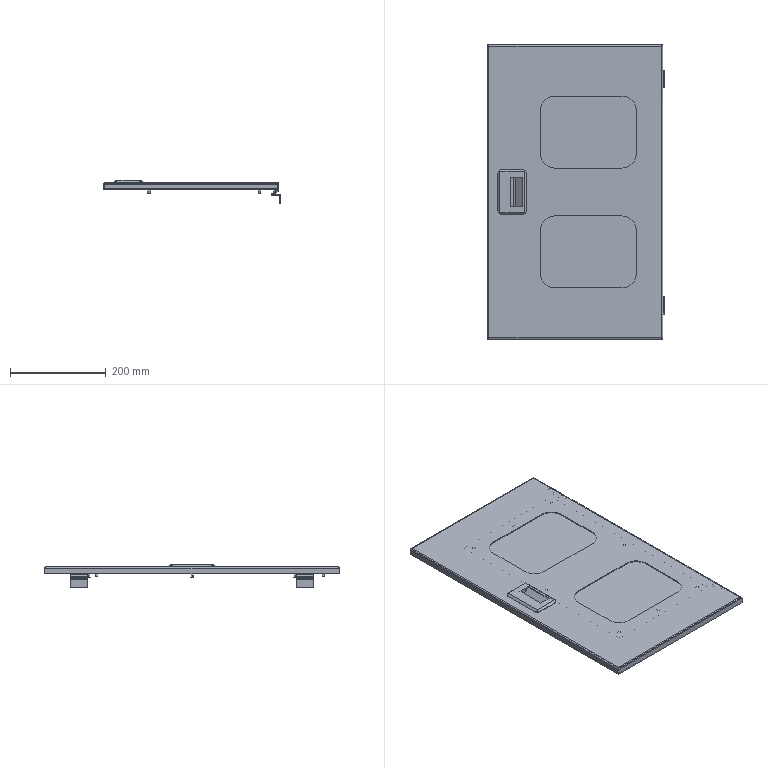Part | SolidWorks | features ReferencePattern 3, CompositeCurve 1, LocalLPattern 1 | 8 solids | 350 faces | box 369.222 x 614 x 49.278 mm | volume 1337700 mm3 | plane 203 | cylinder 139 | cone 8 | commonest cylinder face diameters 7 x28 6 x18 4.5 x16 60 x16 4 x12 5 x12